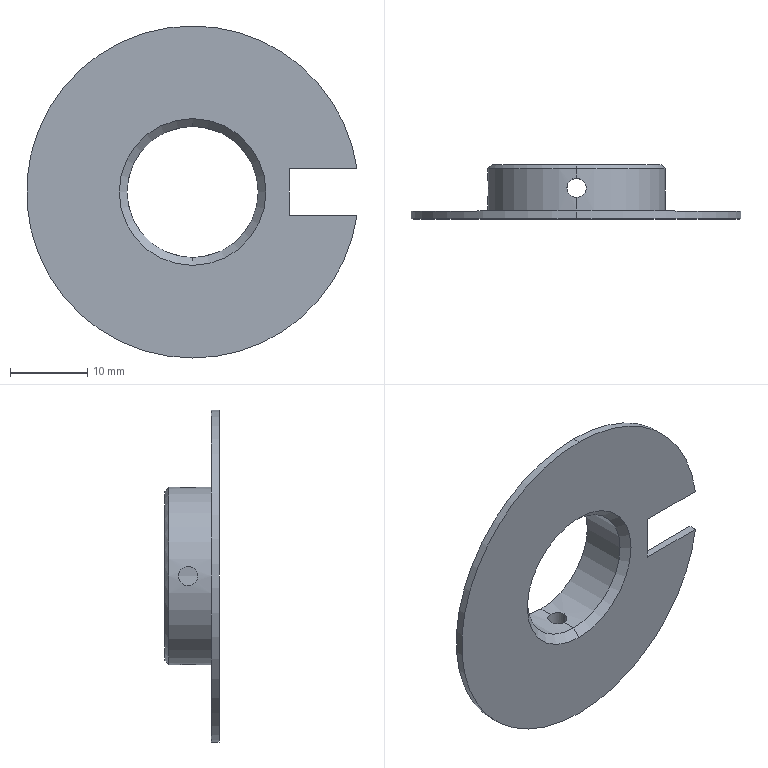Part | SolidWorks | features Chamfer 2, CirPattern 1, HoleWzd 1, ICE 1, Revolution 1 | 1 solid | 23 faces | box 42.79 x 7 x 43 mm | volume 2222 mm3 | cylinder 13 | plane 6 | cone 4 | commonest cylinder face diameters 2.5 x6 43 x3 17 x2 23 x2
STEP:
#1=CARTESIAN_POINT('',(-1.25,4.,-11.432));
#2=VERTEX_POINT('',#1);
#3=CARTESIAN_POINT('',(0.,2.75,-11.5));
#4=VERTEX_POINT('',#3);
#5=CARTESIAN_POINT('',(-1.25,4.,-11.432));
#6=CARTESIAN_POINT('',(-1.25,3.837,-11.432));
#7=CARTESIAN_POINT('',(-1.217,3.672,-11.436));
#8=CARTESIAN_POINT('',(-1.092,3.371,-11.448));
#9=CARTESIAN_POINT('',(-0.9994,3.232,-11.457));
#10=CARTESIAN_POINT('',(-0.7689,3.001,-11.475));
#11=CARTESIAN_POINT('',(-0.6303,2.908,-11.484));
#12=CARTESIAN_POINT('',(-0.3276,2.783,-11.496));
#13=CARTESIAN_POINT('',(-0.1653,2.75,-11.5));
#14=CARTESIAN_POINT('',(0.,2.75,-11.5));
#15=B_SPLINE_CURVE_WITH_KNOTS('',3,(#5,#6,#7,#8,#9,#10,#11,#12,#13,#14),.UNSPECIFIED.,.F.,.F.,(4,2,2,2,4),(0.003911,0.0044,0.004889,0.005378,0.005867),.UNSPECIFIED.);
#16=EDGE_CURVE('',#2,#4,#15,.T.);
#17=ORIENTED_EDGE('',*,*,#16,.F.);
#18=CARTESIAN_POINT('',(-1.25,4.,-8.408));
#19=VERTEX_POINT('',#18);
#20=CARTESIAN_POINT('',(-1.25,4.,0.));
#21=DIRECTION('',(0.,0.,1.));
#22=VECTOR('',#21,1000.);
#23=LINE('',#20,#22);
#24=EDGE_CURVE('',#2,#19,#23,.T.);
#25=ORIENTED_EDGE('',*,*,#24,.T.);
#26=CARTESIAN_POINT('',(0.,2.75,-8.5));
#27=VERTEX_POINT('',#26);
#28=CARTESIAN_POINT('',(0.,2.75,-8.5));
#29=CARTESIAN_POINT('',(-0.08164,2.75,-8.5));
#30=CARTESIAN_POINT('',(-0.1646,2.758,-8.499));
#31=CARTESIAN_POINT('',(-0.3249,2.79,-8.494));
#32=CARTESIAN_POINT('',(-0.4029,2.814,-8.491));
#33=CARTESIAN_POINT('',(-0.63,2.908,-8.478));
#34=CARTESIAN_POINT('',(-0.7675,3.,-8.466));
#35=CARTESIAN_POINT('',(-1.,3.233,-8.442));
#36=CARTESIAN_POINT('',(-1.092,3.37,-8.43));
#37=CARTESIAN_POINT('',(-1.186,3.597,-8.417));
#38=CARTESIAN_POINT('',(-1.21,3.675,-8.413));
#39=CARTESIAN_POINT('',(-1.242,3.835,-8.409));
#40=CARTESIAN_POINT('',(-1.25,3.918,-8.408));
#41=CARTESIAN_POINT('',(-1.25,4.,-8.408));
#42=B_SPLINE_CURVE_WITH_KNOTS('',3,(#28,#29,#30,#31,#32,#33,#34,#35,#36,#37,#38,#39,#40,#41),.UNSPECIFIED.,.F.,.F.,(4,2,2,2,2,2,4),(0.001957,0.002202,0.002446,0.002935,0.003424,0.003669,0.003913),.UNSPECIFIED.);
#43=EDGE_CURVE('',#27,#19,#42,.T.);
#44=ORIENTED_EDGE('',*,*,#43,.F.);
#45=CARTESIAN_POINT('',(1.25,4.,-8.408));
#46=VERTEX_POINT('',#45);
#47=CARTESIAN_POINT('',(1.25,4.,-8.408));
#48=CARTESIAN_POINT('',(1.25,3.835,-8.408));
#49=CARTESIAN_POINT('',(1.217,3.672,-8.413));
#50=CARTESIAN_POINT('',(1.092,3.369,-8.43));
#51=CARTESIAN_POINT('',(0.9988,3.231,-8.442));
#52=CARTESIAN_POINT('',(0.7683,3.001,-8.466));
#53=CARTESIAN_POINT('',(0.6289,2.908,-8.478));
#54=CARTESIAN_POINT('',(0.3281,2.783,-8.495));
#55=CARTESIAN_POINT('',(0.1633,2.75,-8.5));
#56=CARTESIAN_POINT('',(0.,2.75,-8.5));
#57=B_SPLINE_CURVE_WITH_KNOTS('',3,(#47,#48,#49,#50,#51,#52,#53,#54,#55,#56),.UNSPECIFIED.,.F.,.F.,(4,2,2,2,4),(0.,0.0004893,0.0009786,0.001468,0.001957),.UNSPECIFIED.);
#58=EDGE_CURVE('',#46,#27,#57,.T.);
#59=ORIENTED_EDGE('',*,*,#58,.F.);
#60=CARTESIAN_POINT('',(1.25,4.,-11.432));
#61=VERTEX_POINT('',#60);
#62=CARTESIAN_POINT('',(1.25,4.,0.));
#63=DIRECTION('',(0.,0.,1.));
#64=VECTOR('',#63,1000.);
#65=LINE('',#62,#64);
#66=EDGE_CURVE('',#61,#46,#65,.T.);
#67=ORIENTED_EDGE('',*,*,#66,.F.);
#68=CARTESIAN_POINT('',(0.,2.75,-11.5));
#69=CARTESIAN_POINT('',(0.1652,2.75,-11.5));
#70=CARTESIAN_POINT('',(0.3273,2.783,-11.496));
#71=CARTESIAN_POINT('',(0.6299,2.908,-11.484));
#72=CARTESIAN_POINT('',(0.7684,3.001,-11.475));
#73=CARTESIAN_POINT('',(0.9988,3.231,-11.457));
#74=CARTESIAN_POINT('',(1.092,3.37,-11.448));
#75=CARTESIAN_POINT('',(1.217,3.671,-11.436));
#76=CARTESIAN_POINT('',(1.25,3.835,-11.432));
#77=CARTESIAN_POINT('',(1.25,4.,-11.432));
#78=B_SPLINE_CURVE_WITH_KNOTS('',3,(#68,#69,#70,#71,#72,#73,#74,#75,#76,#77),.UNSPECIFIED.,.F.,.F.,(4,2,2,2,4),(0.005867,0.006355,0.006844,0.007332,0.007821),.UNSPECIFIED.);
#79=EDGE_CURVE('',#4,#61,#78,.T.);
#80=ORIENTED_EDGE('',*,*,#79,.F.);
#81=EDGE_LOOP('',(#17,#25,#44,#59,#67,#80));
#82=FACE_OUTER_BOUND('',#81,.T.);
#83=CARTESIAN_POINT('',(0.,4.,0.));
#84=DIRECTION('',(0.,0.,1.));
#85=DIRECTION('',(1.,0.,0.));
#86=AXIS2_PLACEMENT_3D('',#83,#84,#85);
#87=CYLINDRICAL_SURFACE('',#86,1.25);
#88=ADVANCED_FACE('',(#82),#87,.F.);
#89=CARTESIAN_POINT('',(1.25,4.,11.432));
#90=VERTEX_POINT('',#89);
#91=CARTESIAN_POINT('',(0.,2.75,11.5));
#92=VERTEX_POINT('',#91);
#93=CARTESIAN_POINT('',(1.25,4.,11.432));
#94=CARTESIAN_POINT('',(1.25,3.835,11.432));
#95=CARTESIAN_POINT('',(1.217,3.673,11.436));
#96=CARTESIAN_POINT('',(1.092,3.37,11.448));
#97=CARTESIAN_POINT('',(0.9993,3.232,11.457));
#98=CARTESIAN_POINT('',(0.769,3.001,11.475));
#99=CARTESIAN_POINT('',(0.6298,2.908,11.484));
#100=CARTESIAN_POINT('',(0.3293,2.783,11.496));
#101=CARTESIAN_POINT('',(0.1652,2.75,11.5));
#102=CARTESIAN_POINT('',(0.,2.75,11.5));
#103=B_SPLINE_CURVE_WITH_KNOTS('',3,(#93,#94,#95,#96,#97,#98,#99,#100,#101,#102),.UNSPECIFIED.,.F.,.F.,(4,2,2,2,4),(0.005867,0.006355,0.006844,0.007332,0.007821),.UNSPECIFIED.);
#104=EDGE_CURVE('',#90,#92,#103,.T.);
#105=ORIENTED_EDGE('',*,*,#104,.F.);
#106=CARTESIAN_POINT('',(1.25,4.,8.408));
#107=VERTEX_POINT('',#106);
#108=CARTESIAN_POINT('',(1.25,4.,0.));
#109=DIRECTION('',(0.,0.,-1.));
#110=VECTOR('',#109,1000.);
#111=LINE('',#108,#110);
#112=EDGE_CURVE('',#90,#107,#111,.T.);
#113=ORIENTED_EDGE('',*,*,#112,.T.);
#114=CARTESIAN_POINT('',(0.,2.75,8.5));
#115=VERTEX_POINT('',#114);
#116=CARTESIAN_POINT('',(0.,2.75,8.5));
#117=CARTESIAN_POINT('',(0.1655,2.75,8.5));
#118=CARTESIAN_POINT('',(0.3278,2.783,8.495));
#119=CARTESIAN_POINT('',(0.6305,2.908,8.478));
#120=CARTESIAN_POINT('',(0.7691,3.001,8.466));
#121=CARTESIAN_POINT('',(0.9994,3.232,8.442));
#122=CARTESIAN_POINT('',(1.092,3.371,8.43));
#123=CARTESIAN_POINT('',(1.217,3.672,8.413));
#124=CARTESIAN_POINT('',(1.25,3.837,8.408));
#125=CARTESIAN_POINT('',(1.25,4.,8.408));
#126=B_SPLINE_CURVE_WITH_KNOTS('',3,(#116,#117,#118,#119,#120,#121,#122,#123,#124,#125),.UNSPECIFIED.,.F.,.F.,(4,2,2,2,4),(0.,0.0004893,0.0009786,0.001468,0.001957),.UNSPECIFIED.);
#127=EDGE_CURVE('',#115,#107,#126,.T.);
#128=ORIENTED_EDGE('',*,*,#127,.F.);
#129=CARTESIAN_POINT('',(-1.25,4.,8.408));
#130=VERTEX_POINT('',#129);
#131=CARTESIAN_POINT('',(-1.25,4.,8.408));
#132=CARTESIAN_POINT('',(-1.25,3.835,8.408));
#133=CARTESIAN_POINT('',(-1.217,3.672,8.413));
#134=CARTESIAN_POINT('',(-1.092,3.37,8.43));
#135=CARTESIAN_POINT('',(-0.9992,3.232,8.442));
#136=CARTESIAN_POINT('',(-0.7692,3.001,8.466));
#137=CARTESIAN_POINT('',(-0.63,2.908,8.478));
#138=CARTESIAN_POINT('',(-0.3295,2.783,8.495));
#139=CARTESIAN_POINT('',(-0.1653,2.75,8.5));
#140=CARTESIAN_POINT('',(0.,2.75,8.5));
#141=B_SPLINE_CURVE_WITH_KNOTS('',3,(#131,#132,#133,#134,#135,#136,#137,#138,#139,#140),.UNSPECIFIED.,.F.,.F.,(4,2,2,2,4),(0.00587,0.006359,0.006848,0.007337,0.007826),.UNSPECIFIED.);
#142=EDGE_CURVE('',#130,#115,#141,.T.);
#143=ORIENTED_EDGE('',*,*,#142,.F.);
#144=CARTESIAN_POINT('',(-1.25,4.,11.432));
#145=VERTEX_POINT('',#144);
#146=CARTESIAN_POINT('',(-1.25,4.,0.));
#147=DIRECTION('',(0.,0.,-1.));
#148=VECTOR('',#147,1000.);
#149=LINE('',#146,#148);
#150=EDGE_CURVE('',#145,#130,#149,.T.);
#151=ORIENTED_EDGE('',*,*,#150,.F.);
#152=CARTESIAN_POINT('',(0.,2.75,11.5));
#153=CARTESIAN_POINT('',(-0.1654,2.75,11.5));
#154=CARTESIAN_POINT('',(-0.3276,2.783,11.496));
#155=CARTESIAN_POINT('',(-0.6304,2.908,11.484));
#156=CARTESIAN_POINT('',(-0.769,3.001,11.475));
#157=CARTESIAN_POINT('',(-0.9994,3.232,11.457));
#158=CARTESIAN_POINT('',(-1.093,3.371,11.448));
#159=CARTESIAN_POINT('',(-1.217,3.672,11.436));
#160=CARTESIAN_POINT('',(-1.25,3.837,11.432));
#161=CARTESIAN_POINT('',(-1.25,4.,11.432));
#162=B_SPLINE_CURVE_WITH_KNOTS('',3,(#152,#153,#154,#155,#156,#157,#158,#159,#160,#161),.UNSPECIFIED.,.F.,.F.,(4,2,2,2,4),(0.,0.000489,0.000978,0.001467,0.001956),.UNSPECIFIED.);
#163=EDGE_CURVE('',#92,#145,#162,.T.);
#164=ORIENTED_EDGE('',*,*,#163,.F.);
#165=EDGE_LOOP('',(#105,#113,#128,#143,#151,#164));
#166=FACE_OUTER_BOUND('',#165,.T.);
#167=CARTESIAN_POINT('',(0.,4.,0.));
#168=DIRECTION('',(0.,0.,-1.));
#169=DIRECTION('',(-1.,0.,0.));
#170=AXIS2_PLACEMENT_3D('',#167,#168,#169);
#171=CYLINDRICAL_SURFACE('',#170,1.25);
#172=ADVANCED_FACE('',(#166),#171,.F.);
#173=CARTESIAN_POINT('',(0.,7.,11.));
#174=VERTEX_POINT('',#173);
#175=CARTESIAN_POINT('',(0.,7.,-11.));
#176=VERTEX_POINT('',#175);
#177=CARTESIAN_POINT('',(0.,7.,0.));
#178=DIRECTION('',(0.,1.,0.));
#179=DIRECTION('',(0.,0.,-1.));
#180=AXIS2_PLACEMENT_3D('',#177,#178,#179);
#181=CIRCLE('',#180,11.);
#182=EDGE_CURVE('',#174,#176,#181,.T.);
#183=ORIENTED_EDGE('',*,*,#182,.F.);
#184=CARTESIAN_POINT('',(0.,6.5,11.5));
#185=VERTEX_POINT('',#184);
#186=CARTESIAN_POINT('',(0.,7.,11.));
#187=DIRECTION('',(0.,-0.7071,0.7071));
#188=VECTOR('',#187,1000.);
#189=LINE('',#186,#188);
#190=EDGE_CURVE('',#174,#185,#189,.T.);
#191=ORIENTED_EDGE('',*,*,#190,.T.);
#192=CARTESIAN_POINT('',(0.,6.5,-11.5));
#193=VERTEX_POINT('',#192);
#194=CARTESIAN_POINT('',(0.,6.5,0.));
#195=DIRECTION('',(0.,-1.,0.));
#196=DIRECTION('',(0.,0.,-1.));
#197=AXIS2_PLACEMENT_3D('',#194,#195,#196);
#198=CIRCLE('',#197,11.5);
#199=EDGE_CURVE('',#193,#185,#198,.T.);
#200=ORIENTED_EDGE('',*,*,#199,.F.);
#201=CARTESIAN_POINT('',(0.,7.,-11.));
#202=DIRECTION('',(0.,-0.7071,-0.7071));
#203=VECTOR('',#202,1000.);
#204=LINE('',#201,#203);
#205=EDGE_CURVE('',#176,#193,#204,.T.);
#206=ORIENTED_EDGE('',*,*,#205,.F.);
#207=EDGE_LOOP('',(#183,#191,#200,#206));
#208=FACE_OUTER_BOUND('',#207,.T.);
#209=CARTESIAN_POINT('',(0.,7.,0.));
#210=DIRECTION('',(0.,-1.,0.));
#211=DIRECTION('',(0.,0.,-1.));
#212=AXIS2_PLACEMENT_3D('',#209,#210,#211);
#213=CONICAL_SURFACE('',#212,11.,0.7854);
#214=ADVANCED_FACE('',(#208),#213,.T.);
#215=CARTESIAN_POINT('',(-11.432,4.,1.25));
#216=VERTEX_POINT('',#215);
#217=CARTESIAN_POINT('',(-11.432,4.,-1.25));
#218=VERTEX_POINT('',#217);
#219=CARTESIAN_POINT('',(-11.432,4.,1.25));
#220=CARTESIAN_POINT('',(-11.432,3.837,1.25));
#221=CARTESIAN_POINT('',(-11.436,3.672,1.217));
#222=CARTESIAN_POINT('',(-11.448,3.371,1.093));
#223=CARTESIAN_POINT('',(-11.457,3.232,0.9996));
#224=CARTESIAN_POINT('',(-11.475,3.001,0.7693));
#225=CARTESIAN_POINT('',(-11.484,2.909,0.6309));
#226=CARTESIAN_POINT('',(-11.496,2.783,0.3283));
#227=CARTESIAN_POINT('',(-11.5,2.75,0.1661));
#228=CARTESIAN_POINT('',(-11.5,2.75,-0.1643));
#229=CARTESIAN_POINT('',(-11.496,2.782,-0.3265));
#230=CARTESIAN_POINT('',(-11.484,2.908,-0.6294));
#231=CARTESIAN_POINT('',(-11.475,3.,-0.768));
#232=CARTESIAN_POINT('',(-11.457,3.231,-0.9986));
#233=CARTESIAN_POINT('',(-11.448,3.37,-1.092));
#234=CARTESIAN_POINT('',(-11.436,3.671,-1.217));
#235=CARTESIAN_POINT('',(-11.432,3.835,-1.25));
#236=CARTESIAN_POINT('',(-11.432,4.,-1.25));
#237=B_SPLINE_CURVE_WITH_KNOTS('',3,(#219,#220,#221,#222,#223,#224,#225,#226,#227,#228,#229,#230,#231,#232,#233,#234,#235,#236),.UNSPECIFIED.,.F.,.F.,(4,2,2,2,2,2,2,2,4),(0.003911,0.0044,0.004888,0.005377,0.005866,0.006355,0.006843,0.007332,0.007821),.UNSPECIFIED.);
#238=EDGE_CURVE('',#216,#218,#237,.T.);
#239=ORIENTED_EDGE('',*,*,#238,.F.);
#240=CARTESIAN_POINT('',(-8.408,4.,1.25));
#241=VERTEX_POINT('',#240);
#242=CARTESIAN_POINT('',(0.,4.,1.25));
#243=DIRECTION('',(1.,0.,0.));
#244=VECTOR('',#243,1000.);
#245=LINE('',#242,#244);
#246=EDGE_CURVE('',#216,#241,#245,.T.);
#247=ORIENTED_EDGE('',*,*,#246,.T.);
#248=CARTESIAN_POINT('',(-8.408,4.,-1.25));
#249=VERTEX_POINT('',#248);
#250=CARTESIAN_POINT('',(-8.408,4.,-1.25));
#251=CARTESIAN_POINT('',(-8.408,3.835,-1.25));
#252=CARTESIAN_POINT('',(-8.413,3.672,-1.217));
#253=CARTESIAN_POINT('',(-8.43,3.37,-1.092));
#254=CARTESIAN_POINT('',(-8.442,3.231,-0.9989));
#255=CARTESIAN_POINT('',(-8.466,3.001,-0.7685));
#256=CARTESIAN_POINT('',(-8.478,2.908,-0.6292));
#257=CARTESIAN_POINT('',(-8.495,2.783,-0.3284));
#258=CARTESIAN_POINT('',(-8.5,2.75,-0.1638));
#259=CARTESIAN_POINT('',(-8.5,2.75,0.08119));
#260=CARTESIAN_POINT('',(-8.499,2.758,0.1641));
#261=CARTESIAN_POINT('',(-8.494,2.79,0.3246));
#262=CARTESIAN_POINT('',(-8.491,2.814,0.4025));
#263=CARTESIAN_POINT('',(-8.478,2.908,0.6298));
#264=CARTESIAN_POINT('',(-8.466,3.,0.7673));
#265=CARTESIAN_POINT('',(-8.442,3.233,1.));
#266=CARTESIAN_POINT('',(-8.43,3.37,1.092));
#267=CARTESIAN_POINT('',(-8.417,3.597,1.186));
#268=CARTESIAN_POINT('',(-8.413,3.675,1.21));
#269=CARTESIAN_POINT('',(-8.409,3.835,1.242));
#270=CARTESIAN_POINT('',(-8.408,3.918,1.25));
#271=CARTESIAN_POINT('',(-8.408,4.,1.25));
#272=B_SPLINE_CURVE_WITH_KNOTS('',3,(#250,#251,#252,#253,#254,#255,#256,#257,#258,#259,#260,#261,#262,#263,#264,#265,#266,#267,#268,#269,#270,#271),.UNSPECIFIED.,.F.,.F.,(4,2,2,2,2,2,2,2,2,2,4),(0.,0.0004892,0.0009783,0.001468,0.001957,0.002201,0.002446,0.002935,0.003424,0.003669,0.003913),.UNSPECIFIED.);
#273=EDGE_CURVE('',#249,#241,#272,.T.);
#274=ORIENTED_EDGE('',*,*,#273,.F.);
#275=CARTESIAN_POINT('',(0.,4.,-1.25));
#276=DIRECTION('',(1.,0.,0.));
#277=VECTOR('',#276,1000.);
#278=LINE('',#275,#277);
#279=EDGE_CURVE('',#218,#249,#278,.T.);
#280=ORIENTED_EDGE('',*,*,#279,.F.);
#281=EDGE_LOOP('',(#239,#247,#274,#280));
#282=FACE_OUTER_BOUND('',#281,.T.);
#283=CARTESIAN_POINT('',(0.,4.,0.));
#284=DIRECTION('',(1.,0.,0.));
#285=DIRECTION('',(0.,0.,-1.));
#286=AXIS2_PLACEMENT_3D('',#283,#284,#285);
#287=CYLINDRICAL_SURFACE('',#286,1.25);
#288=ADVANCED_FACE('',(#282),#287,.F.);
#289=CARTESIAN_POINT('',(0.,1.,8.5));
#290=VERTEX_POINT('',#289);
#291=CARTESIAN_POINT('',(0.,1.,-8.5));
#292=VERTEX_POINT('',#291);
#293=CARTESIAN_POINT('',(0.,1.,0.));
#294=DIRECTION('',(0.,-1.,0.));
#295=DIRECTION('',(0.,0.,1.));
#296=AXIS2_PLACEMENT_3D('',#293,#294,#295);
#297=CIRCLE('',#296,8.5);
#298=EDGE_CURVE('',#290,#292,#297,.T.);
#299=ORIENTED_EDGE('',*,*,#298,.F.);
#300=CARTESIAN_POINT('',(0.,0.,9.5));
#301=VERTEX_POINT('',#300);
#302=CARTESIAN_POINT('',(0.,0.,9.5));
#303=DIRECTION('',(0.,-0.7071,0.7071));
#304=VECTOR('',#303,1000.);
#305=LINE('',#302,#304);
#306=EDGE_CURVE('',#290,#301,#305,.T.);
#307=ORIENTED_EDGE('',*,*,#306,.T.);
#308=CARTESIAN_POINT('',(0.,0.,-9.5));
#309=VERTEX_POINT('',#308);
#310=CARTESIAN_POINT('',(0.,0.,0.));
#311=DIRECTION('',(0.,1.,0.));
#312=DIRECTION('',(0.,0.,1.));
#313=AXIS2_PLACEMENT_3D('',#310,#311,#312);
#314=CIRCLE('',#313,9.5);
#315=EDGE_CURVE('',#309,#301,#314,.T.);
#316=ORIENTED_EDGE('',*,*,#315,.F.);
#317=CARTESIAN_POINT('',(0.,0.,-9.5));
#318=DIRECTION('',(0.,-0.7071,-0.7071));
#319=VECTOR('',#318,1000.);
#320=LINE('',#317,#319);
#321=EDGE_CURVE('',#292,#309,#320,.T.);
#322=ORIENTED_EDGE('',*,*,#321,.F.);
#323=EDGE_LOOP('',(#299,#307,#316,#322));
#324=FACE_OUTER_BOUND('',#323,.T.);
#325=CARTESIAN_POINT('',(0.,0.,0.));
#326=DIRECTION('',(0.,-1.,0.));
#327=DIRECTION('',(0.,0.,-1.));
#328=AXIS2_PLACEMENT_3D('',#325,#326,#327);
#329=CONICAL_SURFACE('',#328,9.5,0.7854);
#330=ADVANCED_FACE('',(#324),#329,.F.);
#331=ORIENTED_EDGE('',*,*,#273,.T.);
#332=CARTESIAN_POINT('',(-8.408,4.,1.25));
#333=CARTESIAN_POINT('',(-8.408,4.163,1.25));
#334=CARTESIAN_POINT('',(-8.413,4.328,1.217));
#335=CARTESIAN_POINT('',(-8.43,4.629,1.093));
#336=CARTESIAN_POINT('',(-8.442,4.768,0.9996));
#337=CARTESIAN_POINT('',(-8.46,4.941,0.8269));
#338=CARTESIAN_POINT('',(-8.466,4.994,0.7627));
#339=CARTESIAN_POINT('',(-8.477,5.084,0.6271));
#340=CARTESIAN_POINT('',(-8.482,5.123,0.5554));
#341=CARTESIAN_POINT('',(-8.495,5.217,0.3283));
#342=CARTESIAN_POINT('',(-8.5,5.25,0.1661));
#343=CARTESIAN_POINT('',(-8.5,5.25,-0.1644));
#344=CARTESIAN_POINT('',(-8.495,5.218,-0.3269));
#345=CARTESIAN_POINT('',(-8.478,5.092,-0.6294));
#346=CARTESIAN_POINT('',(-8.466,4.999,-0.7681));
#347=CARTESIAN_POINT('',(-8.442,4.769,-0.9985));
#348=CARTESIAN_POINT('',(-8.43,4.63,-1.092));
#349=CARTESIAN_POINT('',(-8.413,4.33,-1.217));
#350=CARTESIAN_POINT('',(-8.408,4.165,-1.25));
#351=CARTESIAN_POINT('',(-8.408,4.,-1.25));
#352=B_SPLINE_CURVE_WITH_KNOTS('',3,(#332,#333,#334,#335,#336,#337,#338,#339,#340,#341,#342,#343,#344,#345,#346,#347,#348,#349,#350,#351),.UNSPECIFIED.,.F.,.F.,(4,2,2,2,2,2,2,2,2,4),(0.003913,0.004402,0.004891,0.005136,0.005381,0.00587,0.006359,0.006848,0.007337,0.007826),.UNSPECIFIED.);
#353=EDGE_CURVE('',#241,#249,#352,.T.);
#354=ORIENTED_EDGE('',*,*,#353,.T.);
#355=EDGE_LOOP('',(#331,#354));
#356=FACE_BOUND('',#355,.T.);
#357=ORIENTED_EDGE('',*,*,#298,.T.);
#358=CARTESIAN_POINT('',(0.,67.295,-8.5));
#359=DIRECTION('',(0.,1.,0.));
#360=VECTOR('',#359,1000.);
#361=LINE('',#358,#360);
#362=EDGE_CURVE('',#292,#27,#361,.T.);
#363=ORIENTED_EDGE('',*,*,#362,.T.);
#364=ORIENTED_EDGE('',*,*,#43,.T.);
#365=CARTESIAN_POINT('',(0.,5.25,-8.5));
#366=VERTEX_POINT('',#365);
#367=CARTESIAN_POINT('',(-1.25,4.,-8.408));
#368=CARTESIAN_POINT('',(-1.25,4.163,-8.408));
#369=CARTESIAN_POINT('',(-1.217,4.328,-8.413));
#370=CARTESIAN_POINT('',(-1.092,4.629,-8.43));
#371=CARTESIAN_POINT('',(-0.9994,4.768,-8.442));
#372=CARTESIAN_POINT('',(-0.8266,4.941,-8.46));
#373=CARTESIAN_POINT('',(-0.7623,4.994,-8.466));
#374=CARTESIAN_POINT('',(-0.6266,5.085,-8.477));
#375=CARTESIAN_POINT('',(-0.5549,5.123,-8.482));
#376=CARTESIAN_POINT('',(-0.3276,5.217,-8.495));
#377=CARTESIAN_POINT('',(-0.1653,5.25,-8.5));
#378=CARTESIAN_POINT('',(0.,5.25,-8.5));
#379=B_SPLINE_CURVE_WITH_KNOTS('',3,(#367,#368,#369,#370,#371,#372,#373,#374,#375,#376,#377,#378),.UNSPECIFIED.,.F.,.F.,(4,2,2,2,2,4),(0.003913,0.004403,0.004892,0.005137,0.005381,0.00587),.UNSPECIFIED.);
#380=EDGE_CURVE('',#19,#366,#379,.T.);
#381=ORIENTED_EDGE('',*,*,#380,.T.);
#382=CARTESIAN_POINT('',(0.,7.,-8.5));
#383=VERTEX_POINT('',#382);
#384=CARTESIAN_POINT('',(0.,67.295,-8.5));
#385=DIRECTION('',(0.,1.,0.));
#386=VECTOR('',#385,1000.);
#387=LINE('',#384,#386);
#388=EDGE_CURVE('',#366,#383,#387,.T.);
#389=ORIENTED_EDGE('',*,*,#388,.T.);
#390=CARTESIAN_POINT('',(0.,7.,8.5));
#391=VERTEX_POINT('',#390);
#392=CARTESIAN_POINT('',(0.,7.,0.));
#393=DIRECTION('',(0.,1.,0.));
#394=DIRECTION('',(0.,0.,1.));
#395=AXIS2_PLACEMENT_3D('',#392,#393,#394);
#396=CIRCLE('',#395,8.5);
#397=EDGE_CURVE('',#383,#391,#396,.T.);
#398=ORIENTED_EDGE('',*,*,#397,.T.);
#399=CARTESIAN_POINT('',(0.,5.25,8.5));
#400=VERTEX_POINT('',#399);
#401=CARTESIAN_POINT('',(0.,67.295,8.5));
#402=DIRECTION('',(0.,1.,0.));
#403=VECTOR('',#402,1000.);
#404=LINE('',#401,#403);
#405=EDGE_CURVE('',#400,#391,#404,.T.);
#406=ORIENTED_EDGE('',*,*,#405,.F.);
#407=CARTESIAN_POINT('',(0.,5.25,8.5));
#408=CARTESIAN_POINT('',(-0.1633,5.25,8.5));
#409=CARTESIAN_POINT('',(-0.328,5.217,8.495));
#410=CARTESIAN_POINT('',(-0.629,5.092,8.478));
#411=CARTESIAN_POINT('',(-0.7683,4.999,8.466));
#412=CARTESIAN_POINT('',(-0.9412,4.827,8.448));
#413=CARTESIAN_POINT('',(-0.994,4.762,8.442));
#414=CARTESIAN_POINT('',(-1.085,4.627,8.431));
#415=CARTESIAN_POINT('',(-1.123,4.555,8.426));
#416=CARTESIAN_POINT('',(-1.217,4.328,8.413));
#417=CARTESIAN_POINT('',(-1.25,4.165,8.408));
#418=CARTESIAN_POINT('',(-1.25,4.,8.408));
#419=B_SPLINE_CURVE_WITH_KNOTS('',3,(#407,#408,#409,#410,#411,#412,#413,#414,#415,#416,#417,#418),.UNSPECIFIED.,.F.,.F.,(4,2,2,2,2,4),(0.003913,0.004403,0.004892,0.005137,0.005381,0.00587),.UNSPECIFIED.);
#420=EDGE_CURVE('',#400,#130,#419,.T.);
#421=ORIENTED_EDGE('',*,*,#420,.T.);
#422=ORIENTED_EDGE('',*,*,#142,.T.);
#423=CARTESIAN_POINT('',(0.,67.295,8.5));
#424=DIRECTION('',(0.,1.,0.));
#425=VECTOR('',#424,1000.);
#426=LINE('',#423,#425);
#427=EDGE_CURVE('',#290,#115,#426,.T.);
#428=ORIENTED_EDGE('',*,*,#427,.F.);
#429=EDGE_LOOP('',(#357,#363,#364,#381,#389,#398,#406,#421,#422,#428));
#430=FACE_OUTER_BOUND('',#429,.T.);
#431=CARTESIAN_POINT('',(0.,67.295,0.));
#432=DIRECTION('',(0.,1.,0.));
#433=DIRECTION('',(0.,0.,1.));
#434=AXIS2_PLACEMENT_3D('',#431,#432,#433);
#435=CYLINDRICAL_SURFACE('',#434,8.5);
#436=ADVANCED_FACE('',(#356,#430),#435,.F.);
#437=CARTESIAN_POINT('',(0.,1.,11.5));
#438=VERTEX_POINT('',#437);
#439=CARTESIAN_POINT('',(0.,1.,-11.5));
#440=VERTEX_POINT('',#439);
#441=CARTESIAN_POINT('',(0.,1.,0.));
#442=DIRECTION('',(0.,1.,0.));
#443=DIRECTION('',(0.,0.,1.));
#444=AXIS2_PLACEMENT_3D('',#441,#442,#443);
#445=CIRCLE('',#444,11.5);
#446=EDGE_CURVE('',#438,#440,#445,.T.);
#447=ORIENTED_EDGE('',*,*,#446,.T.);
#448=CARTESIAN_POINT('',(0.,67.295,-11.5));
#449=DIRECTION('',(0.,1.,0.));
#450=VECTOR('',#449,1000.);
#451=LINE('',#448,#450);
#452=EDGE_CURVE('',#440,#4,#451,.T.);
#453=ORIENTED_EDGE('',*,*,#452,.T.);
#454=ORIENTED_EDGE('',*,*,#79,.T.);
#455=CARTESIAN_POINT('',(0.,5.25,-11.5));
#456=VERTEX_POINT('',#455);
#457=CARTESIAN_POINT('',(1.25,4.,-11.432));
#458=CARTESIAN_POINT('',(1.25,4.165,-11.432));
#459=CARTESIAN_POINT('',(1.217,4.328,-11.436));
#460=CARTESIAN_POINT('',(1.092,4.63,-11.448));
#461=CARTESIAN_POINT('',(0.9989,4.769,-11.457));
#462=CARTESIAN_POINT('',(0.7682,4.999,-11.475));
#463=CARTESIAN_POINT('',(0.6288,5.093,-11.484));
#464=CARTESIAN_POINT('',(0.3279,5.217,-11.496));
#465=CARTESIAN_POINT('',(0.1632,5.25,-11.5));
#466=CARTESIAN_POINT('',(0.,5.25,-11.5));
#467=B_SPLINE_CURVE_WITH_KNOTS('',3,(#457,#458,#459,#460,#461,#462,#463,#464,#465,#466),.UNSPECIFIED.,.F.,.F.,(4,2,2,2,4),(0.,0.000489,0.000978,0.001467,0.001956),.UNSPECIFIED.);
#468=EDGE_CURVE('',#61,#456,#467,.T.);
#469=ORIENTED_EDGE('',*,*,#468,.T.);
#470=CARTESIAN_POINT('',(0.,67.295,-11.5));
#471=DIRECTION('',(0.,1.,0.));
#472=VECTOR('',#471,1000.);
#473=LINE('',#470,#472);
#474=EDGE_CURVE('',#456,#193,#473,.T.);
#475=ORIENTED_EDGE('',*,*,#474,.T.);
#476=ORIENTED_EDGE('',*,*,#199,.T.);
#477=CARTESIAN_POINT('',(0.,5.25,11.5));
#478=VERTEX_POINT('',#477);
#479=CARTESIAN_POINT('',(0.,67.295,11.5));
#480=DIRECTION('',(0.,1.,0.));
#481=VECTOR('',#480,1000.);
#482=LINE('',#479,#481);
#483=EDGE_CURVE('',#478,#185,#482,.T.);
#484=ORIENTED_EDGE('',*,*,#483,.F.);
#485=CARTESIAN_POINT('',(0.,5.25,11.5));
#486=CARTESIAN_POINT('',(0.1633,5.25,11.5));
#487=CARTESIAN_POINT('',(0.3279,5.217,11.496));
#488=CARTESIAN_POINT('',(0.6289,5.092,11.484));
#489=CARTESIAN_POINT('',(0.7683,4.999,11.475));
#490=CARTESIAN_POINT('',(0.9989,4.769,11.457));
#491=CARTESIAN_POINT('',(1.092,4.63,11.448));
#492=CARTESIAN_POINT('',(1.217,4.328,11.436));
#493=CARTESIAN_POINT('',(1.25,4.165,11.432));
#494=CARTESIAN_POINT('',(1.25,4.,11.432));
#495=B_SPLINE_CURVE_WITH_KNOTS('',3,(#485,#486,#487,#488,#489,#490,#491,#492,#493,#494),.UNSPECIFIED.,.F.,.F.,(4,2,2,2,4),(0.003911,0.0044,0.004889,0.005378,0.005867),.UNSPECIFIED.);
#496=EDGE_CURVE('',#478,#90,#495,.T.);
#497=ORIENTED_EDGE('',*,*,#496,.T.);
#498=ORIENTED_EDGE('',*,*,#104,.T.);
#499=CARTESIAN_POINT('',(0.,67.295,11.5));
#500=DIRECTION('',(0.,1.,0.));
#501=VECTOR('',#500,1000.);
#502=LINE('',#499,#501);
#503=EDGE_CURVE('',#438,#92,#502,.T.);
#504=ORIENTED_EDGE('',*,*,#503,.F.);
#505=EDGE_LOOP('',(#447,#453,#454,#469,#475,#476,#484,#497,#498,#504));
#506=FACE_OUTER_BOUND('',#505,.T.);
#507=CARTESIAN_POINT('',(0.,67.295,0.));
#508=DIRECTION('',(0.,1.,0.));
#509=DIRECTION('',(0.,0.,1.));
#510=AXIS2_PLACEMENT_3D('',#507,#508,#509);
#511=CYLINDRICAL_SURFACE('',#510,11.5);
#512=ADVANCED_FACE('',(#506),#511,.T.);
#513=CARTESIAN_POINT('',(21.29,0.,-3.));
#514=VERTEX_POINT('',#513);
#515=CARTESIAN_POINT('',(0.,0.,-21.5));
#516=VERTEX_POINT('',#515);
#517=CARTESIAN_POINT('',(0.,0.,0.));
#518=DIRECTION('',(0.,1.,0.));
#519=DIRECTION('',(0.,0.,1.));
#520=AXIS2_PLACEMENT_3D('',#517,#518,#519);
#521=CIRCLE('',#520,21.5);
#522=EDGE_CURVE('',#514,#516,#521,.T.);
#523=ORIENTED_EDGE('',*,*,#522,.T.);
#524=CARTESIAN_POINT('',(0.,1.,-21.5));
#525=VERTEX_POINT('',#524);
#526=CARTESIAN_POINT('',(0.,67.295,-21.5));
#527=DIRECTION('',(0.,1.,0.));
#528=VECTOR('',#527,1000.);
#529=LINE('',#526,#528);
#530=EDGE_CURVE('',#516,#525,#529,.T.);
#531=ORIENTED_EDGE('',*,*,#530,.T.);
#532=CARTESIAN_POINT('',(21.29,1.,-3.));
#533=VERTEX_POINT('',#532);
#534=CARTESIAN_POINT('',(0.,1.,0.));
#535=DIRECTION('',(0.,1.,0.));
#536=DIRECTION('',(0.,0.,1.));
#537=AXIS2_PLACEMENT_3D('',#534,#535,#536);
#538=CIRCLE('',#537,21.5);
#539=EDGE_CURVE('',#533,#525,#538,.T.);
#540=ORIENTED_EDGE('',*,*,#539,.F.);
#541=CARTESIAN_POINT('',(21.29,67.295,-3.));
#542=DIRECTION('',(0.,-1.,0.));
#543=VECTOR('',#542,1000.);
#544=LINE('',#541,#543);
#545=EDGE_CURVE('',#533,#514,#544,.T.);
#546=ORIENTED_EDGE('',*,*,#545,.T.);
#547=EDGE_LOOP('',(#523,#531,#540,#546));
#548=FACE_OUTER_BOUND('',#547,.T.);
#549=CARTESIAN_POINT('',(0.,67.295,0.));
#550=DIRECTION('',(0.,1.,0.));
#551=DIRECTION('',(0.,0.,1.));
#552=AXIS2_PLACEMENT_3D('',#549,#550,#551);
#553=CYLINDRICAL_SURFACE('',#552,21.5);
#554=ADVANCED_FACE('',(#548),#553,.T.);
#555=ORIENTED_EDGE('',*,*,#530,.F.);
#556=CARTESIAN_POINT('',(0.,0.,21.5));
#557=VERTEX_POINT('',#556);
#558=CARTESIAN_POINT('',(0.,0.,0.));
#559=DIRECTION('',(0.,1.,0.));
#560=DIRECTION('',(0.,0.,1.));
#561=AXIS2_PLACEMENT_3D('',#558,#559,#560);
#562=CIRCLE('',#561,21.5);
#563=EDGE_CURVE('',#516,#557,#562,.T.);
#564=ORIENTED_EDGE('',*,*,#563,.T.);
#565=CARTESIAN_POINT('',(0.,1.,21.5));
#566=VERTEX_POINT('',#565);
#567=CARTESIAN_POINT('',(0.,67.295,21.5));
#568=DIRECTION('',(0.,1.,0.));
#569=VECTOR('',#568,1000.);
#570=LINE('',#567,#569);
#571=EDGE_CURVE('',#557,#566,#570,.T.);
#572=ORIENTED_EDGE('',*,*,#571,.T.);
#573=CARTESIAN_POINT('',(0.,1.,0.));
#574=DIRECTION('',(0.,1.,0.));
#575=DIRECTION('',(0.,0.,1.));
#576=AXIS2_PLACEMENT_3D('',#573,#574,#575);
#577=CIRCLE('',#576,21.5);
#578=EDGE_CURVE('',#525,#566,#577,.T.);
#579=ORIENTED_EDGE('',*,*,#578,.F.);
#580=EDGE_LOOP('',(#555,#564,#572,#579));
#581=FACE_OUTER_BOUND('',#580,.T.);
#582=CARTESIAN_POINT('',(0.,67.295,0.));
#583=DIRECTION('',(0.,1.,0.));
#584=DIRECTION('',(0.,0.,1.));
#585=AXIS2_PLACEMENT_3D('',#582,#583,#584);
#586=CYLINDRICAL_SURFACE('',#585,21.5);
#587=ADVANCED_FACE('',(#581),#586,.T.);
#588=ORIENTED_EDGE('',*,*,#571,.F.);
#589=CARTESIAN_POINT('',(21.29,0.,3.));
#590=VERTEX_POINT('',#589);
#591=CARTESIAN_POINT('',(0.,0.,0.));
#592=DIRECTION('',(0.,1.,0.));
#593=DIRECTION('',(0.,0.,1.));
#594=AXIS2_PLACEMENT_3D('',#591,#592,#593);
#595=CIRCLE('',#594,21.5);
#596=EDGE_CURVE('',#557,#590,#595,.T.);
#597=ORIENTED_EDGE('',*,*,#596,.T.);
#598=CARTESIAN_POINT('',(21.29,1.,3.));
#599=VERTEX_POINT('',#598);
#600=CARTESIAN_POINT('',(21.29,67.295,3.));
#601=DIRECTION('',(0.,1.,0.));
#602=VECTOR('',#601,1000.);
#603=LINE('',#600,#602);
#604=EDGE_CURVE('',#590,#599,#603,.T.);
#605=ORIENTED_EDGE('',*,*,#604,.T.);
#606=CARTESIAN_POINT('',(0.,1.,0.));
#607=DIRECTION('',(0.,1.,0.));
#608=DIRECTION('',(0.,0.,1.));
#609=AXIS2_PLACEMENT_3D('',#606,#607,#608);
#610=CIRCLE('',#609,21.5);
#611=EDGE_CURVE('',#566,#599,#610,.T.);
#612=ORIENTED_EDGE('',*,*,#611,.F.);
#613=EDGE_LOOP('',(#588,#597,#605,#612));
#614=FACE_OUTER_BOUND('',#613,.T.);
#615=CARTESIAN_POINT('',(0.,67.295,0.));
#616=DIRECTION('',(0.,1.,0.));
#617=DIRECTION('',(0.,0.,1.));
#618=AXIS2_PLACEMENT_3D('',#615,#616,#617);
#619=CYLINDRICAL_SURFACE('',#618,21.5);
#620=ADVANCED_FACE('',(#614),#619,.T.);
#621=ORIENTED_EDGE('',*,*,#446,.F.);
#622=CARTESIAN_POINT('',(0.,1.,0.));
#623=DIRECTION('',(0.,1.,0.));
#624=DIRECTION('',(0.,0.,1.));
#625=AXIS2_PLACEMENT_3D('',#622,#623,#624);
#626=CIRCLE('',#625,11.5);
#627=EDGE_CURVE('',#440,#438,#626,.T.);
#628=ORIENTED_EDGE('',*,*,#627,.F.);
#629=EDGE_LOOP('',(#621,#628));
#630=FACE_BOUND('',#629,.T.);
#631=CARTESIAN_POINT('',(12.5,1.,-3.));
#632=VERTEX_POINT('',#631);
#633=CARTESIAN_POINT('',(12.5,1.,3.));
#634=VERTEX_POINT('',#633);
#635=CARTESIAN_POINT('',(12.5,1.,-3.));
#636=DIRECTION('',(0.,0.,1.));
#637=VECTOR('',#636,1000.);
#638=LINE('',#635,#637);
#639=EDGE_CURVE('',#632,#634,#638,.T.);
#640=ORIENTED_EDGE('',*,*,#639,.F.);
#641=CARTESIAN_POINT('',(12.5,1.,-3.));
#642=DIRECTION('',(-1.,0.,0.));
#643=VECTOR('',#642,1000.);
#644=LINE('',#641,#643);
#645=EDGE_CURVE('',#533,#632,#644,.T.);
#646=ORIENTED_EDGE('',*,*,#645,.F.);
#647=ORIENTED_EDGE('',*,*,#539,.T.);
#648=ORIENTED_EDGE('',*,*,#578,.T.);
#649=ORIENTED_EDGE('',*,*,#611,.T.);
#650=CARTESIAN_POINT('',(12.5,1.,3.));
#651=DIRECTION('',(1.,0.,0.));
#652=VECTOR('',#651,1000.);
#653=LINE('',#650,#652);
#654=EDGE_CURVE('',#634,#599,#653,.T.);
#655=ORIENTED_EDGE('',*,*,#654,.F.);
#656=EDGE_LOOP('',(#640,#646,#647,#648,#649,#655));
#657=FACE_OUTER_BOUND('',#656,.T.);
#658=CARTESIAN_POINT('',(0.,1.,-21.5));
#659=DIRECTION('',(0.,-1.,0.));
#660=DIRECTION('',(0.,0.,-1.));
#661=AXIS2_PLACEMENT_3D('',#658,#659,#660);
#662=PLANE('',#661);
#663=ADVANCED_FACE('',(#630,#657),#662,.F.);
#664=ORIENTED_EDGE('',*,*,#452,.F.);
#665=ORIENTED_EDGE('',*,*,#627,.T.);
#666=ORIENTED_EDGE('',*,*,#503,.T.);
#667=ORIENTED_EDGE('',*,*,#163,.T.);
#668=CARTESIAN_POINT('',(-1.25,4.,11.432));
#669=CARTESIAN_POINT('',(-1.25,4.082,11.432));
#670=CARTESIAN_POINT('',(-1.242,4.164,11.433));
#671=CARTESIAN_POINT('',(-1.21,4.325,11.436));
#672=CARTESIAN_POINT('',(-1.186,4.403,11.439));
#673=CARTESIAN_POINT('',(-1.092,4.63,11.448));
#674=CARTESIAN_POINT('',(-1.001,4.767,11.457));
#675=CARTESIAN_POINT('',(-0.7672,5.001,11.475));
#676=CARTESIAN_POINT('',(-0.6297,5.092,11.484));
#677=CARTESIAN_POINT('',(-0.4027,5.186,11.493));
#678=CARTESIAN_POINT('',(-0.3247,5.21,11.496));
#679=CARTESIAN_POINT('',(-0.1645,5.242,11.499));
#680=CARTESIAN_POINT('',(-0.08159,5.25,11.5));
#681=CARTESIAN_POINT('',(0.,5.25,11.5));
#682=B_SPLINE_CURVE_WITH_KNOTS('',3,(#668,#669,#670,#671,#672,#673,#674,#675,#676,#677,#678,#679,#680,#681),.UNSPECIFIED.,.F.,.F.,(4,2,2,2,2,2,4),(0.001956,0.0022,0.002445,0.002933,0.003422,0.003667,0.003911),.UNSPECIFIED.);
#683=EDGE_CURVE('',#145,#478,#682,.T.);
#684=ORIENTED_EDGE('',*,*,#683,.T.);
#685=ORIENTED_EDGE('',*,*,#483,.T.);
#686=CARTESIAN_POINT('',(0.,6.5,0.));
#687=DIRECTION('',(0.,-1.,0.));
#688=DIRECTION('',(0.,0.,-1.));
#689=AXIS2_PLACEMENT_3D('',#686,#687,#688);
#690=CIRCLE('',#689,11.5);
#691=EDGE_CURVE('',#185,#193,#690,.T.);
#692=ORIENTED_EDGE('',*,*,#691,.T.);
#693=ORIENTED_EDGE('',*,*,#474,.F.);
#694=CARTESIAN_POINT('',(0.,5.25,-11.5));
#695=CARTESIAN_POINT('',(-0.08158,5.25,-11.5));
#696=CARTESIAN_POINT('',(-0.1644,5.242,-11.499));
#697=CARTESIAN_POINT('',(-0.3248,5.21,-11.496));
#698=CARTESIAN_POINT('',(-0.4027,5.186,-11.493));
#699=CARTESIAN_POINT('',(-0.6297,5.092,-11.484));
#700=CARTESIAN_POINT('',(-0.7673,5.001,-11.475));
#701=CARTESIAN_POINT('',(-1.001,4.767,-11.457));
#702=CARTESIAN_POINT('',(-1.092,4.63,-11.448));
#703=CARTESIAN_POINT('',(-1.186,4.403,-11.439));
#704=CARTESIAN_POINT('',(-1.21,4.325,-11.436));
#705=CARTESIAN_POINT('',(-1.242,4.164,-11.433));
#706=CARTESIAN_POINT('',(-1.25,4.082,-11.432));
#707=CARTESIAN_POINT('',(-1.25,4.,-11.432));
#708=B_SPLINE_CURVE_WITH_KNOTS('',3,(#694,#695,#696,#697,#698,#699,#700,#701,#702,#703,#704,#705,#706,#707),.UNSPECIFIED.,.F.,.F.,(4,2,2,2,2,2,4),(0.001956,0.0022,0.002445,0.002933,0.003422,0.003667,0.003911),.UNSPECIFIED.);
#709=EDGE_CURVE('',#456,#2,#708,.T.);
#710=ORIENTED_EDGE('',*,*,#709,.T.);
#711=ORIENTED_EDGE('',*,*,#16,.T.);
#712=EDGE_LOOP('',(#664,#665,#666,#667,#684,#685,#692,#693,#710,#711));
#713=FACE_OUTER_BOUND('',#712,.T.);
#714=CARTESIAN_POINT('',(-11.432,4.,-1.25));
#715=CARTESIAN_POINT('',(-11.432,4.165,-1.25));
#716=CARTESIAN_POINT('',(-11.436,4.328,-1.217));
#717=CARTESIAN_POINT('',(-11.448,4.63,-1.092));
#718=CARTESIAN_POINT('',(-11.457,4.769,-0.999));
#719=CARTESIAN_POINT('',(-11.475,4.999,-0.7685));
#720=CARTESIAN_POINT('',(-11.484,5.092,-0.6291));
#721=CARTESIAN_POINT('',(-11.496,5.217,-0.3282));
#722=CARTESIAN_POINT('',(-11.5,5.25,-0.1636));
#723=CARTESIAN_POINT('',(-11.5,5.25,0.08114));
#724=CARTESIAN_POINT('',(-11.499,5.242,0.164));
#725=CARTESIAN_POINT('',(-11.496,5.21,0.3244));
#726=CARTESIAN_POINT('',(-11.493,5.186,0.4024));
#727=CARTESIAN_POINT('',(-11.484,5.092,0.6295));
#728=CARTESIAN_POINT('',(-11.475,5.001,0.7671));
#729=CARTESIAN_POINT('',(-11.457,4.767,1.));
#730=CARTESIAN_POINT('',(-11.448,4.63,1.092));
#731=CARTESIAN_POINT('',(-11.439,4.403,1.186));
#732=CARTESIAN_POINT('',(-11.436,4.325,1.21));
#733=CARTESIAN_POINT('',(-11.433,4.165,1.242));
#734=CARTESIAN_POINT('',(-11.432,4.082,1.25));
#735=CARTESIAN_POINT('',(-11.432,4.,1.25));
#736=B_SPLINE_CURVE_WITH_KNOTS('',3,(#714,#715,#716,#717,#718,#719,#720,#721,#722,#723,#724,#725,#726,#727,#728,#729,#730,#731,#732,#733,#734,#735),.UNSPECIFIED.,.F.,.F.,(4,2,2,2,2,2,2,2,2,2,4),(0.,0.0004889,0.0009777,0.001467,0.001955,0.0022,0.002444,0.002933,0.003422,0.003667,0.003911),.UNSPECIFIED.);
#737=EDGE_CURVE('',#218,#216,#736,.T.);
#738=ORIENTED_EDGE('',*,*,#737,.T.);
#739=ORIENTED_EDGE('',*,*,#238,.T.);
#740=EDGE_LOOP('',(#738,#739));
#741=FACE_BOUND('',#740,.T.);
#742=CARTESIAN_POINT('',(0.,67.295,0.));
#743=DIRECTION('',(0.,1.,0.));
#744=DIRECTION('',(0.,0.,1.));
#745=AXIS2_PLACEMENT_3D('',#742,#743,#744);
#746=CYLINDRICAL_SURFACE('',#745,11.5);
#747=ADVANCED_FACE('',(#713,#741),#746,.T.);
#748=CARTESIAN_POINT('',(0.,7.,0.));
#749=DIRECTION('',(0.,1.,0.));
#750=DIRECTION('',(0.,0.,-1.));
#751=AXIS2_PLACEMENT_3D('',#748,#749,#750);
#752=CIRCLE('',#751,11.);
#753=EDGE_CURVE('',#176,#174,#752,.T.);
#754=ORIENTED_EDGE('',*,*,#753,.T.);
#755=ORIENTED_EDGE('',*,*,#182,.T.);
#756=EDGE_LOOP('',(#754,#755));
#757=FACE_OUTER_BOUND('',#756,.T.);
#758=CARTESIAN_POINT('',(0.,7.,0.));
#759=DIRECTION('',(0.,1.,0.));
#760=DIRECTION('',(0.,0.,1.));
#761=AXIS2_PLACEMENT_3D('',#758,#759,#760);
#762=CIRCLE('',#761,8.5);
#763=EDGE_CURVE('',#391,#383,#762,.T.);
#764=ORIENTED_EDGE('',*,*,#763,.F.);
#765=ORIENTED_EDGE('',*,*,#397,.F.);
#766=EDGE_LOOP('',(#764,#765));
#767=FACE_BOUND('',#766,.T.);
#768=CARTESIAN_POINT('',(0.,7.,-11.5));
#769=DIRECTION('',(0.,-1.,0.));
#770=DIRECTION('',(0.,0.,-1.));
#771=AXIS2_PLACEMENT_3D('',#768,#769,#770);
#772=PLANE('',#771);
#773=ADVANCED_FACE('',(#757,#767),#772,.F.);
#774=ORIENTED_EDGE('',*,*,#362,.F.);
#775=CARTESIAN_POINT('',(0.,1.,0.));
#776=DIRECTION('',(0.,-1.,0.));
#777=DIRECTION('',(0.,0.,1.));
#778=AXIS2_PLACEMENT_3D('',#775,#776,#777);
#779=CIRCLE('',#778,8.5);
#780=EDGE_CURVE('',#292,#290,#779,.T.);
#781=ORIENTED_EDGE('',*,*,#780,.T.);
#782=ORIENTED_EDGE('',*,*,#427,.T.);
#783=ORIENTED_EDGE('',*,*,#127,.T.);
#784=CARTESIAN_POINT('',(1.25,4.,8.408));
#785=CARTESIAN_POINT('',(1.25,4.082,8.408));
#786=CARTESIAN_POINT('',(1.242,4.165,8.409));
#787=CARTESIAN_POINT('',(1.21,4.325,8.413));
#788=CARTESIAN_POINT('',(1.186,4.403,8.417));
#789=CARTESIAN_POINT('',(1.092,4.63,8.43));
#790=CARTESIAN_POINT('',(1.,4.768,8.442));
#791=CARTESIAN_POINT('',(0.7673,5.,8.466));
#792=CARTESIAN_POINT('',(0.6297,5.092,8.478));
#793=CARTESIAN_POINT('',(0.4028,5.186,8.491));
#794=CARTESIAN_POINT('',(0.3249,5.21,8.494));
#795=CARTESIAN_POINT('',(0.1645,5.242,8.499));
#796=CARTESIAN_POINT('',(0.08162,5.25,8.5));
#797=CARTESIAN_POINT('',(0.,5.25,8.5));
#798=B_SPLINE_CURVE_WITH_KNOTS('',3,(#784,#785,#786,#787,#788,#789,#790,#791,#792,#793,#794,#795,#796,#797),.UNSPECIFIED.,.F.,.F.,(4,2,2,2,2,2,4),(0.001957,0.002202,0.002446,0.002935,0.003424,0.003669,0.003913),.UNSPECIFIED.);
#799=EDGE_CURVE('',#107,#400,#798,.T.);
#800=ORIENTED_EDGE('',*,*,#799,.T.);
#801=ORIENTED_EDGE('',*,*,#405,.T.);
#802=ORIENTED_EDGE('',*,*,#763,.T.);
#803=ORIENTED_EDGE('',*,*,#388,.F.);
#804=CARTESIAN_POINT('',(0.,5.25,-8.5));
#805=CARTESIAN_POINT('',(0.1651,5.25,-8.5));
#806=CARTESIAN_POINT('',(0.3276,5.217,-8.495));
#807=CARTESIAN_POINT('',(0.6299,5.092,-8.478));
#808=CARTESIAN_POINT('',(0.7685,4.999,-8.466));
#809=CARTESIAN_POINT('',(0.9987,4.769,-8.442));
#810=CARTESIAN_POINT('',(1.092,4.63,-8.43));
#811=CARTESIAN_POINT('',(1.217,4.33,-8.413));
#812=CARTESIAN_POINT('',(1.25,4.165,-8.408));
#813=CARTESIAN_POINT('',(1.25,4.,-8.408));
#814=B_SPLINE_CURVE_WITH_KNOTS('',3,(#804,#805,#806,#807,#808,#809,#810,#811,#812,#813),.UNSPECIFIED.,.F.,.F.,(4,2,2,2,4),(0.00587,0.006359,0.006848,0.007337,0.007826),.UNSPECIFIED.);
#815=EDGE_CURVE('',#366,#46,#814,.T.);
#816=ORIENTED_EDGE('',*,*,#815,.T.);
#817=ORIENTED_EDGE('',*,*,#58,.T.);
#818=EDGE_LOOP('',(#774,#781,#782,#783,#800,#801,#802,#803,#816,#817));
#819=FACE_OUTER_BOUND('',#818,.T.);
#820=CARTESIAN_POINT('',(0.,67.295,0.));
#821=DIRECTION('',(0.,1.,0.));
#822=DIRECTION('',(0.,0.,1.));
#823=AXIS2_PLACEMENT_3D('',#820,#821,#822);
#824=CYLINDRICAL_SURFACE('',#823,8.5);
#825=ADVANCED_FACE('',(#819),#824,.F.);
#826=ORIENTED_EDGE('',*,*,#315,.T.);
#827=CARTESIAN_POINT('',(0.,0.,0.));
#828=DIRECTION('',(0.,1.,0.));
#829=DIRECTION('',(0.,0.,1.));
#830=AXIS2_PLACEMENT_3D('',#827,#828,#829);
#831=CIRCLE('',#830,9.5);
#832=EDGE_CURVE('',#301,#309,#831,.T.);
#833=ORIENTED_EDGE('',*,*,#832,.T.);
#834=EDGE_LOOP('',(#826,#833));
#835=FACE_BOUND('',#834,.T.);
#836=ORIENTED_EDGE('',*,*,#522,.F.);
#837=CARTESIAN_POINT('',(12.5,0.,-3.));
#838=VERTEX_POINT('',#837);
#839=CARTESIAN_POINT('',(0.,0.,-3.));
#840=DIRECTION('',(-1.,0.,0.));
#841=VECTOR('',#840,1000.);
#842=LINE('',#839,#841);
#843=EDGE_CURVE('',#514,#838,#842,.T.);
#844=ORIENTED_EDGE('',*,*,#843,.T.);
#845=CARTESIAN_POINT('',(12.5,0.,3.));
#846=VERTEX_POINT('',#845);
#847=CARTESIAN_POINT('',(12.5,0.,-8.5));
#848=DIRECTION('',(0.,0.,1.));
#849=VECTOR('',#848,1000.);
#850=LINE('',#847,#849);
#851=EDGE_CURVE('',#838,#846,#850,.T.);
#852=ORIENTED_EDGE('',*,*,#851,.T.);
#853=CARTESIAN_POINT('',(0.,0.,3.));
#854=DIRECTION('',(1.,0.,0.));
#855=VECTOR('',#854,1000.);
#856=LINE('',#853,#855);
#857=EDGE_CURVE('',#846,#590,#856,.T.);
#858=ORIENTED_EDGE('',*,*,#857,.T.);
#859=ORIENTED_EDGE('',*,*,#596,.F.);
#860=ORIENTED_EDGE('',*,*,#563,.F.);
#861=EDGE_LOOP('',(#836,#844,#852,#858,#859,#860));
#862=FACE_OUTER_BOUND('',#861,.T.);
#863=CARTESIAN_POINT('',(0.,0.,-8.5));
#864=DIRECTION('',(0.,1.,0.));
#865=DIRECTION('',(0.,0.,1.));
#866=AXIS2_PLACEMENT_3D('',#863,#864,#865);
#867=PLANE('',#866);
#868=ADVANCED_FACE('',(#835,#862),#867,.F.);
#869=ORIENTED_EDGE('',*,*,#306,.F.);
#870=ORIENTED_EDGE('',*,*,#780,.F.);
#871=ORIENTED_EDGE('',*,*,#321,.T.);
#872=ORIENTED_EDGE('',*,*,#832,.F.);
#873=EDGE_LOOP('',(#869,#870,#871,#872));
#874=FACE_OUTER_BOUND('',#873,.T.);
#875=CARTESIAN_POINT('',(0.,0.,0.));
#876=DIRECTION('',(0.,-1.,0.));
#877=DIRECTION('',(0.,0.,-1.));
#878=AXIS2_PLACEMENT_3D('',#875,#876,#877);
#879=CONICAL_SURFACE('',#878,9.5,0.7854);
#880=ADVANCED_FACE('',(#874),#879,.F.);
#881=CARTESIAN_POINT('',(12.5,-9.,-3.));
#882=DIRECTION('',(0.,1.,0.));
#883=VECTOR('',#882,1000.);
#884=LINE('',#881,#883);
#885=EDGE_CURVE('',#838,#632,#884,.T.);
#886=ORIENTED_EDGE('',*,*,#885,.T.);
#887=ORIENTED_EDGE('',*,*,#639,.T.);
#888=CARTESIAN_POINT('',(12.5,-9.,3.));
#889=DIRECTION('',(0.,1.,0.));
#890=VECTOR('',#889,1000.);
#891=LINE('',#888,#890);
#892=EDGE_CURVE('',#846,#634,#891,.T.);
#893=ORIENTED_EDGE('',*,*,#892,.F.);
#894=ORIENTED_EDGE('',*,*,#851,.F.);
#895=EDGE_LOOP('',(#886,#887,#893,#894));
#896=FACE_OUTER_BOUND('',#895,.T.);
#897=CARTESIAN_POINT('',(12.5,-9.,-3.));
#898=DIRECTION('',(-1.,0.,0.));
#899=DIRECTION('',(0.,0.,1.));
#900=AXIS2_PLACEMENT_3D('',#897,#898,#899);
#901=PLANE('',#900);
#902=ADVANCED_FACE('',(#896),#901,.F.);
#903=ORIENTED_EDGE('',*,*,#645,.T.);
#904=ORIENTED_EDGE('',*,*,#885,.F.);
#905=ORIENTED_EDGE('',*,*,#843,.F.);
#906=ORIENTED_EDGE('',*,*,#545,.F.);
#907=EDGE_LOOP('',(#903,#904,#905,#906));
#908=FACE_OUTER_BOUND('',#907,.T.);
#909=CARTESIAN_POINT('',(12.5,-9.,-3.));
#910=DIRECTION('',(0.,0.,-1.));
#911=DIRECTION('',(-1.,0.,0.));
#912=AXIS2_PLACEMENT_3D('',#909,#910,#911);
#913=PLANE('',#912);
#914=ADVANCED_FACE('',(#908),#913,.F.);
#915=ORIENTED_EDGE('',*,*,#857,.F.);
#916=ORIENTED_EDGE('',*,*,#892,.T.);
#917=ORIENTED_EDGE('',*,*,#654,.T.);
#918=ORIENTED_EDGE('',*,*,#604,.F.);
#919=EDGE_LOOP('',(#915,#916,#917,#918));
#920=FACE_OUTER_BOUND('',#919,.T.);
#921=CARTESIAN_POINT('',(12.5,-9.,3.));
#922=DIRECTION('',(0.,0.,1.));
#923=DIRECTION('',(1.,0.,0.));
#924=AXIS2_PLACEMENT_3D('',#921,#922,#923);
#925=PLANE('',#924);
#926=ADVANCED_FACE('',(#920),#925,.F.);
#927=ORIENTED_EDGE('',*,*,#246,.F.);
#928=ORIENTED_EDGE('',*,*,#737,.F.);
#929=ORIENTED_EDGE('',*,*,#279,.T.);
#930=ORIENTED_EDGE('',*,*,#353,.F.);
#931=EDGE_LOOP('',(#927,#928,#929,#930));
#932=FACE_OUTER_BOUND('',#931,.T.);
#933=CARTESIAN_POINT('',(0.,4.,0.));
#934=DIRECTION('',(1.,0.,0.));
#935=DIRECTION('',(0.,0.,-1.));
#936=AXIS2_PLACEMENT_3D('',#933,#934,#935);
#937=CYLINDRICAL_SURFACE('',#936,1.25);
#938=ADVANCED_FACE('',(#932),#937,.F.);
#939=ORIENTED_EDGE('',*,*,#190,.F.);
#940=ORIENTED_EDGE('',*,*,#753,.F.);
#941=ORIENTED_EDGE('',*,*,#205,.T.);
#942=ORIENTED_EDGE('',*,*,#691,.F.);
#943=EDGE_LOOP('',(#939,#940,#941,#942));
#944=FACE_OUTER_BOUND('',#943,.T.);
#945=CARTESIAN_POINT('',(0.,7.,0.));
#946=DIRECTION('',(0.,-1.,0.));
#947=DIRECTION('',(0.,0.,-1.));
#948=AXIS2_PLACEMENT_3D('',#945,#946,#947);
#949=CONICAL_SURFACE('',#948,11.,0.7854);
#950=ADVANCED_FACE('',(#944),#949,.T.);
#951=ORIENTED_EDGE('',*,*,#112,.F.);
#952=ORIENTED_EDGE('',*,*,#496,.F.);
#953=ORIENTED_EDGE('',*,*,#683,.F.);
#954=ORIENTED_EDGE('',*,*,#150,.T.);
#955=ORIENTED_EDGE('',*,*,#420,.F.);
#956=ORIENTED_EDGE('',*,*,#799,.F.);
#957=EDGE_LOOP('',(#951,#952,#953,#954,#955,#956));
#958=FACE_OUTER_BOUND('',#957,.T.);
#959=CARTESIAN_POINT('',(0.,4.,0.));
#960=DIRECTION('',(0.,0.,-1.));
#961=DIRECTION('',(-1.,0.,0.));
#962=AXIS2_PLACEMENT_3D('',#959,#960,#961);
#963=CYLINDRICAL_SURFACE('',#962,1.25);
#964=ADVANCED_FACE('',(#958),#963,.F.);
#965=ORIENTED_EDGE('',*,*,#24,.F.);
#966=ORIENTED_EDGE('',*,*,#709,.F.);
#967=ORIENTED_EDGE('',*,*,#468,.F.);
#968=ORIENTED_EDGE('',*,*,#66,.T.);
#969=ORIENTED_EDGE('',*,*,#815,.F.);
#970=ORIENTED_EDGE('',*,*,#380,.F.);
#971=EDGE_LOOP('',(#965,#966,#967,#968,#969,#970));
#972=FACE_OUTER_BOUND('',#971,.T.);
#973=CARTESIAN_POINT('',(0.,4.,0.));
#974=DIRECTION('',(0.,0.,1.));
#975=DIRECTION('',(1.,0.,0.));
#976=AXIS2_PLACEMENT_3D('',#973,#974,#975);
#977=CYLINDRICAL_SURFACE('',#976,1.25);
#978=ADVANCED_FACE('',(#972),#977,.F.);
#979=CLOSED_SHELL('',(#88,#172,#214,#288,#330,#436,#512,#554,#587,#620,#663,#747,#773,#825,#868,#880,#902,#914,#926,#938,#950,#964,#978));
#980=MANIFOLD_SOLID_BREP('',#979);
#981=CARTESIAN_POINT('',(0.,0.,0.));
#982=DIRECTION('',(0.,0.,1.));
#983=DIRECTION('',(1.,0.,0.));
#984=AXIS2_PLACEMENT_3D('',#981,#982,#983);
#985=(LENGTH_UNIT()NAMED_UNIT(*)SI_UNIT(.MILLI.,.METRE.));
#986=UNCERTAINTY_MEASURE_WITH_UNIT(LENGTH_MEASURE(0.00001),#985,'','');
#987=(NAMED_UNIT(*)PLANE_ANGLE_UNIT()SI_UNIT($,.RADIAN.));
#988=(NAMED_UNIT(*)SI_UNIT($,.STERADIAN.)SOLID_ANGLE_UNIT());
#989=(GEOMETRIC_REPRESENTATION_CONTEXT(3)GLOBAL_UNCERTAINTY_ASSIGNED_CONTEXT((#986))GLOBAL_UNIT_ASSIGNED_CONTEXT((#985,#987,#988))REPRESENTATION_CONTEXT('',''));
#990=ADVANCED_BREP_SHAPE_REPRESENTATION('',(#980,#984),#989);